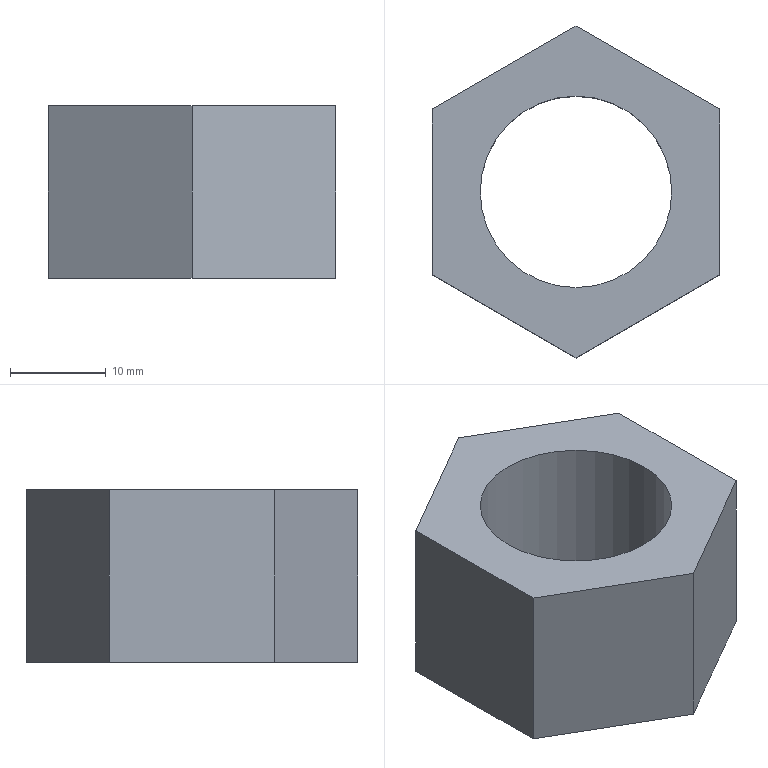Part | NX | features solid 2 | 1 solid | 9 faces | box 30 x 34.641 x 18 mm | volume 8375 mm3 | plane 8 | cylinder 1 | commonest cylinder face diameters 20 x1
STEP:
#1=CARTESIAN_POINT('',(652.5,-157.321,-53.));
#2=VERTEX_POINT('',#1);
#3=CARTESIAN_POINT('',(637.5,-148.66,-53.));
#4=VERTEX_POINT('',#3);
#5=CARTESIAN_POINT('',(652.5,-157.321,-53.));
#6=DIRECTION('',(-0.866,0.5,0.));
#7=VECTOR('',#6,1000.);
#8=LINE('',#5,#7);
#9=EDGE_CURVE('',#2,#4,#8,.T.);
#10=ORIENTED_EDGE('',*,*,#9,.F.);
#11=CARTESIAN_POINT('',(652.5,-157.321,-35.));
#12=VERTEX_POINT('',#11);
#13=CARTESIAN_POINT('',(652.5,-157.321,-35.));
#14=DIRECTION('',(0.,0.,-1.));
#15=VECTOR('',#14,1000.);
#16=LINE('',#13,#15);
#17=EDGE_CURVE('',#12,#2,#16,.T.);
#18=ORIENTED_EDGE('',*,*,#17,.F.);
#19=CARTESIAN_POINT('',(637.5,-148.66,-35.));
#20=VERTEX_POINT('',#19);
#21=CARTESIAN_POINT('',(652.5,-157.321,-35.));
#22=DIRECTION('',(-0.866,0.5,0.));
#23=VECTOR('',#22,1000.);
#24=LINE('',#21,#23);
#25=EDGE_CURVE('',#12,#20,#24,.T.);
#26=ORIENTED_EDGE('',*,*,#25,.T.);
#27=CARTESIAN_POINT('',(637.5,-148.66,-35.));
#28=DIRECTION('',(0.,0.,-1.));
#29=VECTOR('',#28,1000.);
#30=LINE('',#27,#29);
#31=EDGE_CURVE('',#20,#4,#30,.T.);
#32=ORIENTED_EDGE('',*,*,#31,.T.);
#33=EDGE_LOOP('',(#10,#18,#26,#32));
#34=FACE_BOUND('',#33,.T.);
#35=CARTESIAN_POINT('',(652.5,-157.321,-35.));
#36=DIRECTION('',(0.5,0.866,0.));
#37=DIRECTION('',(0.866,-0.5,0.));
#38=AXIS2_PLACEMENT_3D('',#35,#36,#37);
#39=PLANE('',#38);
#40=ADVANCED_FACE('',(#34),#39,.F.);
#41=CARTESIAN_POINT('',(637.5,-131.34,-53.));
#42=VERTEX_POINT('',#41);
#43=CARTESIAN_POINT('',(637.5,-148.66,-53.));
#44=DIRECTION('',(0.,1.,0.));
#45=VECTOR('',#44,1000.);
#46=LINE('',#43,#45);
#47=EDGE_CURVE('',#4,#42,#46,.T.);
#48=ORIENTED_EDGE('',*,*,#47,.F.);
#49=ORIENTED_EDGE('',*,*,#31,.F.);
#50=CARTESIAN_POINT('',(637.5,-131.34,-35.));
#51=VERTEX_POINT('',#50);
#52=CARTESIAN_POINT('',(637.5,-148.66,-35.));
#53=DIRECTION('',(0.,1.,0.));
#54=VECTOR('',#53,1000.);
#55=LINE('',#52,#54);
#56=EDGE_CURVE('',#20,#51,#55,.T.);
#57=ORIENTED_EDGE('',*,*,#56,.T.);
#58=CARTESIAN_POINT('',(637.5,-131.34,-35.));
#59=DIRECTION('',(0.,0.,-1.));
#60=VECTOR('',#59,1000.);
#61=LINE('',#58,#60);
#62=EDGE_CURVE('',#51,#42,#61,.T.);
#63=ORIENTED_EDGE('',*,*,#62,.T.);
#64=EDGE_LOOP('',(#48,#49,#57,#63));
#65=FACE_BOUND('',#64,.T.);
#66=CARTESIAN_POINT('',(637.5,-148.66,-35.));
#67=DIRECTION('',(1.,0.,0.));
#68=DIRECTION('',(0.,-1.,0.));
#69=AXIS2_PLACEMENT_3D('',#66,#67,#68);
#70=PLANE('',#69);
#71=ADVANCED_FACE('',(#65),#70,.F.);
#72=CARTESIAN_POINT('',(652.5,-122.679,-53.));
#73=VERTEX_POINT('',#72);
#74=CARTESIAN_POINT('',(637.5,-131.34,-53.));
#75=DIRECTION('',(0.866,0.5,0.));
#76=VECTOR('',#75,1000.);
#77=LINE('',#74,#76);
#78=EDGE_CURVE('',#42,#73,#77,.T.);
#79=ORIENTED_EDGE('',*,*,#78,.F.);
#80=ORIENTED_EDGE('',*,*,#62,.F.);
#81=CARTESIAN_POINT('',(652.5,-122.679,-35.));
#82=VERTEX_POINT('',#81);
#83=CARTESIAN_POINT('',(637.5,-131.34,-35.));
#84=DIRECTION('',(0.866,0.5,0.));
#85=VECTOR('',#84,1000.);
#86=LINE('',#83,#85);
#87=EDGE_CURVE('',#51,#82,#86,.T.);
#88=ORIENTED_EDGE('',*,*,#87,.T.);
#89=CARTESIAN_POINT('',(652.5,-122.679,-35.));
#90=DIRECTION('',(0.,0.,-1.));
#91=VECTOR('',#90,1000.);
#92=LINE('',#89,#91);
#93=EDGE_CURVE('',#82,#73,#92,.T.);
#94=ORIENTED_EDGE('',*,*,#93,.T.);
#95=EDGE_LOOP('',(#79,#80,#88,#94));
#96=FACE_BOUND('',#95,.T.);
#97=CARTESIAN_POINT('',(637.5,-131.34,-35.));
#98=DIRECTION('',(0.5,-0.866,0.));
#99=DIRECTION('',(-0.866,-0.5,0.));
#100=AXIS2_PLACEMENT_3D('',#97,#98,#99);
#101=PLANE('',#100);
#102=ADVANCED_FACE('',(#96),#101,.F.);
#103=CARTESIAN_POINT('',(667.5,-131.34,-53.));
#104=VERTEX_POINT('',#103);
#105=CARTESIAN_POINT('',(652.5,-122.679,-53.));
#106=DIRECTION('',(0.866,-0.5,0.));
#107=VECTOR('',#106,1000.);
#108=LINE('',#105,#107);
#109=EDGE_CURVE('',#73,#104,#108,.T.);
#110=ORIENTED_EDGE('',*,*,#109,.F.);
#111=ORIENTED_EDGE('',*,*,#93,.F.);
#112=CARTESIAN_POINT('',(667.5,-131.34,-35.));
#113=VERTEX_POINT('',#112);
#114=CARTESIAN_POINT('',(652.5,-122.679,-35.));
#115=DIRECTION('',(0.866,-0.5,0.));
#116=VECTOR('',#115,1000.);
#117=LINE('',#114,#116);
#118=EDGE_CURVE('',#82,#113,#117,.T.);
#119=ORIENTED_EDGE('',*,*,#118,.T.);
#120=CARTESIAN_POINT('',(667.5,-131.34,-35.));
#121=DIRECTION('',(0.,0.,-1.));
#122=VECTOR('',#121,1000.);
#123=LINE('',#120,#122);
#124=EDGE_CURVE('',#113,#104,#123,.T.);
#125=ORIENTED_EDGE('',*,*,#124,.T.);
#126=EDGE_LOOP('',(#110,#111,#119,#125));
#127=FACE_BOUND('',#126,.T.);
#128=CARTESIAN_POINT('',(652.5,-122.679,-35.));
#129=DIRECTION('',(-0.5,-0.866,0.));
#130=DIRECTION('',(-0.866,0.5,0.));
#131=AXIS2_PLACEMENT_3D('',#128,#129,#130);
#132=PLANE('',#131);
#133=ADVANCED_FACE('',(#127),#132,.F.);
#134=CARTESIAN_POINT('',(667.5,-148.66,-53.));
#135=VERTEX_POINT('',#134);
#136=CARTESIAN_POINT('',(667.5,-131.34,-53.));
#137=DIRECTION('',(0.,-1.,0.));
#138=VECTOR('',#137,1000.);
#139=LINE('',#136,#138);
#140=EDGE_CURVE('',#104,#135,#139,.T.);
#141=ORIENTED_EDGE('',*,*,#140,.F.);
#142=ORIENTED_EDGE('',*,*,#124,.F.);
#143=CARTESIAN_POINT('',(667.5,-148.66,-35.));
#144=VERTEX_POINT('',#143);
#145=CARTESIAN_POINT('',(667.5,-131.34,-35.));
#146=DIRECTION('',(0.,-1.,0.));
#147=VECTOR('',#146,1000.);
#148=LINE('',#145,#147);
#149=EDGE_CURVE('',#113,#144,#148,.T.);
#150=ORIENTED_EDGE('',*,*,#149,.T.);
#151=CARTESIAN_POINT('',(667.5,-148.66,-35.));
#152=DIRECTION('',(0.,0.,-1.));
#153=VECTOR('',#152,1000.);
#154=LINE('',#151,#153);
#155=EDGE_CURVE('',#144,#135,#154,.T.);
#156=ORIENTED_EDGE('',*,*,#155,.T.);
#157=EDGE_LOOP('',(#141,#142,#150,#156));
#158=FACE_BOUND('',#157,.T.);
#159=CARTESIAN_POINT('',(667.5,-131.34,-35.));
#160=DIRECTION('',(-1.,0.,0.));
#161=DIRECTION('',(0.,1.,0.));
#162=AXIS2_PLACEMENT_3D('',#159,#160,#161);
#163=PLANE('',#162);
#164=ADVANCED_FACE('',(#158),#163,.F.);
#165=CARTESIAN_POINT('',(652.5,-150.,-35.));
#166=VERTEX_POINT('',#165);
#167=CARTESIAN_POINT('',(652.5,-140.,-35.));
#168=DIRECTION('',(0.,0.,1.));
#169=DIRECTION('',(0.,-1.,0.));
#170=AXIS2_PLACEMENT_3D('',#167,#168,#169);
#171=CIRCLE('',#170,10.);
#172=EDGE_CURVE('',#166,#166,#171,.F.);
#173=ORIENTED_EDGE('',*,*,#172,.F.);
#174=EDGE_LOOP('',(#173));
#175=FACE_BOUND('',#174,.T.);
#176=CARTESIAN_POINT('',(652.5,-150.,-53.));
#177=VERTEX_POINT('',#176);
#178=CARTESIAN_POINT('',(652.5,-140.,-53.));
#179=DIRECTION('',(0.,0.,1.));
#180=DIRECTION('',(0.,-1.,0.));
#181=AXIS2_PLACEMENT_3D('',#178,#179,#180);
#182=CIRCLE('',#181,10.);
#183=EDGE_CURVE('',#177,#177,#182,.F.);
#184=ORIENTED_EDGE('',*,*,#183,.T.);
#185=EDGE_LOOP('',(#184));
#186=FACE_BOUND('',#185,.T.);
#187=CARTESIAN_POINT('',(652.5,-140.,-24.));
#188=DIRECTION('',(0.,0.,-1.));
#189=DIRECTION('',(0.,-1.,0.));
#190=AXIS2_PLACEMENT_3D('',#187,#188,#189);
#191=CYLINDRICAL_SURFACE('',#190,10.);
#192=ADVANCED_FACE('',(#175,#186),#191,.F.);
#193=CARTESIAN_POINT('',(667.5,-148.66,-53.));
#194=DIRECTION('',(-0.866,-0.5,0.));
#195=VECTOR('',#194,1000.);
#196=LINE('',#193,#195);
#197=EDGE_CURVE('',#135,#2,#196,.T.);
#198=ORIENTED_EDGE('',*,*,#197,.F.);
#199=ORIENTED_EDGE('',*,*,#155,.F.);
#200=CARTESIAN_POINT('',(667.5,-148.66,-35.));
#201=DIRECTION('',(-0.866,-0.5,0.));
#202=VECTOR('',#201,1000.);
#203=LINE('',#200,#202);
#204=EDGE_CURVE('',#144,#12,#203,.T.);
#205=ORIENTED_EDGE('',*,*,#204,.T.);
#206=ORIENTED_EDGE('',*,*,#17,.T.);
#207=EDGE_LOOP('',(#198,#199,#205,#206));
#208=FACE_BOUND('',#207,.T.);
#209=CARTESIAN_POINT('',(667.5,-148.66,-35.));
#210=DIRECTION('',(-0.5,0.866,0.));
#211=DIRECTION('',(0.866,0.5,0.));
#212=AXIS2_PLACEMENT_3D('',#209,#210,#211);
#213=PLANE('',#212);
#214=ADVANCED_FACE('',(#208),#213,.F.);
#215=ORIENTED_EDGE('',*,*,#172,.T.);
#216=EDGE_LOOP('',(#215));
#217=FACE_BOUND('',#216,.T.);
#218=ORIENTED_EDGE('',*,*,#25,.F.);
#219=ORIENTED_EDGE('',*,*,#204,.F.);
#220=ORIENTED_EDGE('',*,*,#149,.F.);
#221=ORIENTED_EDGE('',*,*,#118,.F.);
#222=ORIENTED_EDGE('',*,*,#87,.F.);
#223=ORIENTED_EDGE('',*,*,#56,.F.);
#224=EDGE_LOOP('',(#218,#219,#220,#221,#222,#223));
#225=FACE_BOUND('',#224,.T.);
#226=CARTESIAN_POINT('',(667.5,-165.981,-35.));
#227=DIRECTION('',(0.,0.,-1.));
#228=DIRECTION('',(0.,-1.,0.));
#229=AXIS2_PLACEMENT_3D('',#226,#227,#228);
#230=PLANE('',#229);
#231=ADVANCED_FACE('',(#217,#225),#230,.F.);
#232=ORIENTED_EDGE('',*,*,#183,.F.);
#233=EDGE_LOOP('',(#232));
#234=FACE_BOUND('',#233,.T.);
#235=ORIENTED_EDGE('',*,*,#9,.T.);
#236=ORIENTED_EDGE('',*,*,#47,.T.);
#237=ORIENTED_EDGE('',*,*,#78,.T.);
#238=ORIENTED_EDGE('',*,*,#109,.T.);
#239=ORIENTED_EDGE('',*,*,#140,.T.);
#240=ORIENTED_EDGE('',*,*,#197,.T.);
#241=EDGE_LOOP('',(#235,#236,#237,#238,#239,#240));
#242=FACE_BOUND('',#241,.T.);
#243=CARTESIAN_POINT('',(667.5,-165.981,-53.));
#244=DIRECTION('',(0.,0.,-1.));
#245=DIRECTION('',(0.,-1.,0.));
#246=AXIS2_PLACEMENT_3D('',#243,#244,#245);
#247=PLANE('',#246);
#248=ADVANCED_FACE('',(#234,#242),#247,.T.);
#249=CLOSED_SHELL('',(#40,#71,#102,#133,#164,#192,#214,#231,#248));
#250=MANIFOLD_SOLID_BREP('',#249);
#251=(LENGTH_UNIT()NAMED_UNIT(*)SI_UNIT(.MILLI.,.METRE.));
#252=UNCERTAINTY_MEASURE_WITH_UNIT(LENGTH_MEASURE(0.00001),#251,'','');
#253=(NAMED_UNIT(*)PLANE_ANGLE_UNIT()SI_UNIT($,.RADIAN.));
#254=(NAMED_UNIT(*)SI_UNIT($,.STERADIAN.)SOLID_ANGLE_UNIT());
#255=(GEOMETRIC_REPRESENTATION_CONTEXT(3)GLOBAL_UNCERTAINTY_ASSIGNED_CONTEXT((#252))GLOBAL_UNIT_ASSIGNED_CONTEXT((#251,#253,#254))REPRESENTATION_CONTEXT('',''));
#256=ADVANCED_BREP_SHAPE_REPRESENTATION('',(#250),#255);